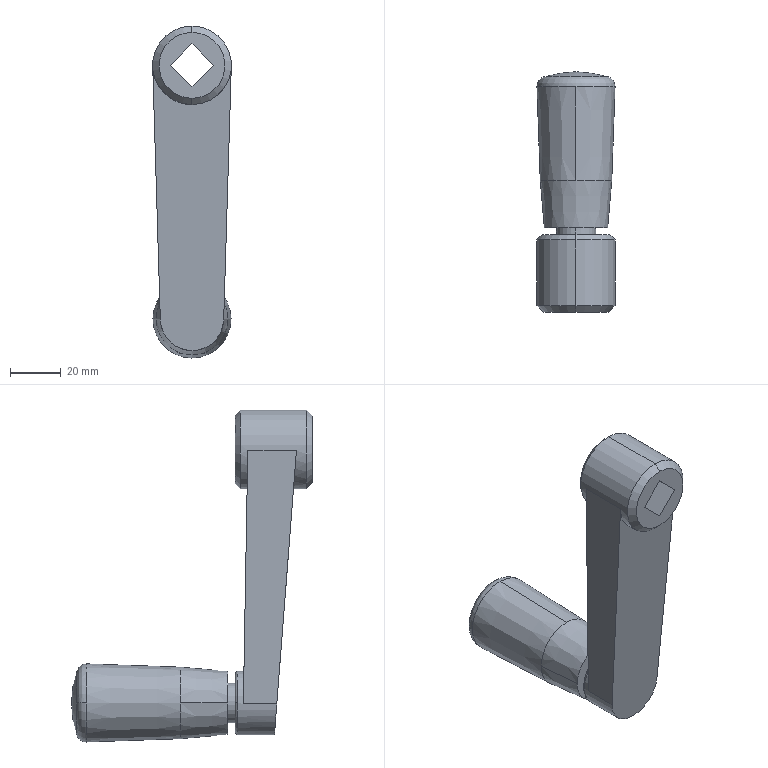Part | SolidWorks | features BaseBody 1 | 1 solid | 34 faces | box 31 x 95 x 130.902 mm | volume 100335 mm3 | plane 13 | cylinder 8 | cone 8 | torus 4 | sphere 1 | commonest cylinder face diameters 15.5 x2 19.799 x2 25 x2 31 x2
STEP:
#1=CARTESIAN_POINT('',(12.494,13.56,-100.375));
#2=VERTEX_POINT('',#1);
#3=CARTESIAN_POINT('',(0.,14.5,-112.5));
#4=VERTEX_POINT('',#3);
#5=CARTESIAN_POINT('',(12.494,13.56,-100.375));
#6=CARTESIAN_POINT('',(12.28,14.114,-107.521));
#7=CARTESIAN_POINT('',(7.149,14.5,-112.5));
#8=CARTESIAN_POINT('',(0.,14.5,-112.5));
#9=(BOUNDED_CURVE()B_SPLINE_CURVE(3,(#5,#6,#7,#8),.UNSPECIFIED.,.F.,.F.)B_SPLINE_CURVE_WITH_KNOTS((4,4),(4.742,6.283),.UNSPECIFIED.)CURVE()GEOMETRIC_REPRESENTATION_ITEM()RATIONAL_B_SPLINE_CURVE((1.,0.8118,0.8118,1.))REPRESENTATION_ITEM(''));
#10=EDGE_CURVE('',#2,#4,#9,.T.);
#11=ORIENTED_EDGE('',*,*,#10,.T.);
#12=CARTESIAN_POINT('',(0.,29.,-112.5));
#13=VERTEX_POINT('',#12);
#14=CARTESIAN_POINT('',(0.,30.,-112.5));
#15=DIRECTION('',(0.,1.,0.));
#16=VECTOR('',#15,1000.);
#17=LINE('',#14,#16);
#18=EDGE_CURVE('',#4,#13,#17,.T.);
#19=ORIENTED_EDGE('',*,*,#18,.T.);
#20=CARTESIAN_POINT('',(12.5,29.,-100.));
#21=VERTEX_POINT('',#20);
#22=CARTESIAN_POINT('',(0.,29.,-100.));
#23=DIRECTION('',(0.,-1.,0.));
#24=DIRECTION('',(0.,0.,1.));
#25=AXIS2_PLACEMENT_3D('',#22,#23,#24);
#26=CIRCLE('',#25,12.5);
#27=EDGE_CURVE('',#13,#21,#26,.T.);
#28=ORIENTED_EDGE('',*,*,#27,.T.);
#29=CARTESIAN_POINT('',(0.,29.,-87.5));
#30=VERTEX_POINT('',#29);
#31=CARTESIAN_POINT('',(0.,29.,-100.));
#32=DIRECTION('',(0.,-1.,0.));
#33=DIRECTION('',(0.,0.,1.));
#34=AXIS2_PLACEMENT_3D('',#31,#32,#33);
#35=CIRCLE('',#34,12.5);
#36=EDGE_CURVE('',#21,#30,#35,.T.);
#37=ORIENTED_EDGE('',*,*,#36,.T.);
#38=CARTESIAN_POINT('',(0.,26.527,-87.5));
#39=VERTEX_POINT('',#38);
#40=CARTESIAN_POINT('',(0.,30.,-87.5));
#41=DIRECTION('',(0.,1.,0.));
#42=VECTOR('',#41,1000.);
#43=LINE('',#40,#42);
#44=EDGE_CURVE('',#39,#30,#43,.T.);
#45=ORIENTED_EDGE('',*,*,#44,.F.);
#46=CARTESIAN_POINT('',(12.494,26.752,-100.375));
#47=VERTEX_POINT('',#46);
#48=CARTESIAN_POINT('',(0.,26.527,-87.5));
#49=CARTESIAN_POINT('',(7.498,26.527,-87.5));
#50=CARTESIAN_POINT('',(12.719,26.621,-92.881));
#51=CARTESIAN_POINT('',(12.494,26.752,-100.375));
#52=(BOUNDED_CURVE()B_SPLINE_CURVE(3,(#48,#49,#50,#51),.UNSPECIFIED.,.F.,.F.)B_SPLINE_CURVE_WITH_KNOTS((4,4),(3.142,4.742),.UNSPECIFIED.)CURVE()GEOMETRIC_REPRESENTATION_ITEM()RATIONAL_B_SPLINE_CURVE((1.,0.7976,0.7976,1.))REPRESENTATION_ITEM(''));
#53=EDGE_CURVE('',#39,#47,#52,.T.);
#54=ORIENTED_EDGE('',*,*,#53,.T.);
#55=CARTESIAN_POINT('',(12.494,30.,-100.375));
#56=DIRECTION('',(0.,-1.,0.));
#57=VECTOR('',#56,1000.);
#58=LINE('',#55,#57);
#59=EDGE_CURVE('',#47,#2,#58,.T.);
#60=ORIENTED_EDGE('',*,*,#59,.T.);
#61=EDGE_LOOP('',(#11,#19,#28,#37,#45,#54,#60));
#62=FACE_OUTER_BOUND('',#61,.T.);
#63=CARTESIAN_POINT('',(0.,30.,-100.));
#64=DIRECTION('',(0.,1.,0.));
#65=DIRECTION('',(0.,0.,1.));
#66=AXIS2_PLACEMENT_3D('',#63,#64,#65);
#67=CYLINDRICAL_SURFACE('',#66,12.5);
#68=ADVANCED_FACE('',(#62),#67,.T.);
#69=CARTESIAN_POINT('',(0.,2.,15.5));
#70=VERTEX_POINT('',#69);
#71=CARTESIAN_POINT('',(0.,2.,-15.5));
#72=VERTEX_POINT('',#71);
#73=CARTESIAN_POINT('',(0.,2.,0.));
#74=DIRECTION('',(0.,1.,0.));
#75=DIRECTION('',(0.,0.,1.));
#76=AXIS2_PLACEMENT_3D('',#73,#74,#75);
#77=CIRCLE('',#76,15.5);
#78=EDGE_CURVE('',#70,#72,#77,.T.);
#79=ORIENTED_EDGE('',*,*,#78,.T.);
#80=CARTESIAN_POINT('',(0.,6.98,-15.5));
#81=VERTEX_POINT('',#80);
#82=CARTESIAN_POINT('',(0.,30.,-15.5));
#83=DIRECTION('',(0.,1.,0.));
#84=VECTOR('',#83,1000.);
#85=LINE('',#82,#84);
#86=EDGE_CURVE('',#72,#81,#85,.T.);
#87=ORIENTED_EDGE('',*,*,#86,.T.);
#88=CARTESIAN_POINT('',(15.493,5.815,-0.465));
#89=VERTEX_POINT('',#88);
#90=CARTESIAN_POINT('',(0.,6.98,-15.5));
#91=CARTESIAN_POINT('',(8.865,6.98,-15.5));
#92=CARTESIAN_POINT('',(15.227,6.502,-9.326));
#93=CARTESIAN_POINT('',(15.493,5.815,-0.465));
#94=(BOUNDED_CURVE()B_SPLINE_CURVE(3,(#90,#91,#92,#93),.UNSPECIFIED.,.F.,.F.)B_SPLINE_CURVE_WITH_KNOTS((4,4),(0.,1.541),.UNSPECIFIED.)CURVE()GEOMETRIC_REPRESENTATION_ITEM()RATIONAL_B_SPLINE_CURVE((1.,0.8118,0.8118,1.))REPRESENTATION_ITEM(''));
#95=EDGE_CURVE('',#81,#89,#94,.T.);
#96=ORIENTED_EDGE('',*,*,#95,.T.);
#97=CARTESIAN_POINT('',(15.493,25.008,-0.465));
#98=VERTEX_POINT('',#97);
#99=CARTESIAN_POINT('',(15.493,30.,-0.465));
#100=DIRECTION('',(0.,1.,0.));
#101=VECTOR('',#100,1000.);
#102=LINE('',#99,#101);
#103=EDGE_CURVE('',#89,#98,#102,.T.);
#104=ORIENTED_EDGE('',*,*,#103,.T.);
#105=CARTESIAN_POINT('',(0.,25.271,-15.5));
#106=VERTEX_POINT('',#105);
#107=CARTESIAN_POINT('',(15.493,25.008,-0.465));
#108=CARTESIAN_POINT('',(15.227,25.163,-9.326));
#109=CARTESIAN_POINT('',(8.865,25.271,-15.5));
#110=CARTESIAN_POINT('',(0.,25.271,-15.5));
#111=(BOUNDED_CURVE()B_SPLINE_CURVE(3,(#107,#108,#109,#110),.UNSPECIFIED.,.F.,.F.)B_SPLINE_CURVE_WITH_KNOTS((4,4),(4.742,6.283),.UNSPECIFIED.)CURVE()GEOMETRIC_REPRESENTATION_ITEM()RATIONAL_B_SPLINE_CURVE((1.,0.8118,0.8118,1.))REPRESENTATION_ITEM(''));
#112=EDGE_CURVE('',#98,#106,#111,.T.);
#113=ORIENTED_EDGE('',*,*,#112,.T.);
#114=CARTESIAN_POINT('',(0.,28.,-15.5));
#115=VERTEX_POINT('',#114);
#116=CARTESIAN_POINT('',(0.,30.,-15.5));
#117=DIRECTION('',(0.,1.,0.));
#118=VECTOR('',#117,1000.);
#119=LINE('',#116,#118);
#120=EDGE_CURVE('',#106,#115,#119,.T.);
#121=ORIENTED_EDGE('',*,*,#120,.T.);
#122=CARTESIAN_POINT('',(0.,28.,15.5));
#123=VERTEX_POINT('',#122);
#124=CARTESIAN_POINT('',(0.,28.,0.));
#125=DIRECTION('',(0.,-1.,0.));
#126=DIRECTION('',(0.,0.,1.));
#127=AXIS2_PLACEMENT_3D('',#124,#125,#126);
#128=CIRCLE('',#127,15.5);
#129=EDGE_CURVE('',#115,#123,#128,.T.);
#130=ORIENTED_EDGE('',*,*,#129,.T.);
#131=CARTESIAN_POINT('',(0.,30.,15.5));
#132=DIRECTION('',(0.,1.,0.));
#133=VECTOR('',#132,1000.);
#134=LINE('',#131,#133);
#135=EDGE_CURVE('',#70,#123,#134,.T.);
#136=ORIENTED_EDGE('',*,*,#135,.F.);
#137=EDGE_LOOP('',(#79,#87,#96,#104,#113,#121,#130,#136));
#138=FACE_OUTER_BOUND('',#137,.T.);
#139=CARTESIAN_POINT('',(0.,30.,0.));
#140=DIRECTION('',(0.,1.,0.));
#141=DIRECTION('',(0.,0.,1.));
#142=AXIS2_PLACEMENT_3D('',#139,#140,#141);
#143=CYLINDRICAL_SURFACE('',#142,15.5);
#144=ADVANCED_FACE('',(#138),#143,.T.);
#145=CARTESIAN_POINT('',(0.,30.,-88.5));
#146=VERTEX_POINT('',#145);
#147=CARTESIAN_POINT('',(-11.5,30.,-100.));
#148=VERTEX_POINT('',#147);
#149=CARTESIAN_POINT('',(0.,30.,-100.));
#150=DIRECTION('',(0.,-1.,0.));
#151=DIRECTION('',(1.,0.,0.));
#152=AXIS2_PLACEMENT_3D('',#149,#150,#151);
#153=CIRCLE('',#152,11.5);
#154=EDGE_CURVE('',#146,#148,#153,.T.);
#155=ORIENTED_EDGE('',*,*,#154,.T.);
#156=CARTESIAN_POINT('',(-12.5,29.,-100.));
#157=VERTEX_POINT('',#156);
#158=CARTESIAN_POINT('',(-11.5,29.,-100.));
#159=DIRECTION('',(0.,0.,1.));
#160=DIRECTION('',(1.,0.,0.));
#161=AXIS2_PLACEMENT_3D('',#158,#159,#160);
#162=CIRCLE('',#161,1.);
#163=EDGE_CURVE('',#148,#157,#162,.T.);
#164=ORIENTED_EDGE('',*,*,#163,.T.);
#165=CARTESIAN_POINT('',(0.,29.,-100.));
#166=DIRECTION('',(0.,-1.,0.));
#167=DIRECTION('',(0.,0.,1.));
#168=AXIS2_PLACEMENT_3D('',#165,#166,#167);
#169=CIRCLE('',#168,12.5);
#170=EDGE_CURVE('',#30,#157,#169,.T.);
#171=ORIENTED_EDGE('',*,*,#170,.F.);
#172=ORIENTED_EDGE('',*,*,#36,.F.);
#173=CARTESIAN_POINT('',(11.5,30.,-100.));
#174=VERTEX_POINT('',#173);
#175=CARTESIAN_POINT('',(11.5,29.,-100.));
#176=DIRECTION('',(0.,0.,-1.));
#177=DIRECTION('',(0.,1.,0.));
#178=AXIS2_PLACEMENT_3D('',#175,#176,#177);
#179=CIRCLE('',#178,1.);
#180=EDGE_CURVE('',#174,#21,#179,.T.);
#181=ORIENTED_EDGE('',*,*,#180,.F.);
#182=CARTESIAN_POINT('',(11.5,30.,-100.));
#183=CARTESIAN_POINT('',(11.5,30.,-98.495));
#184=CARTESIAN_POINT('',(11.201,30.,-96.99));
#185=CARTESIAN_POINT('',(10.049,30.,-94.208));
#186=CARTESIAN_POINT('',(9.196,30.,-92.933));
#187=CARTESIAN_POINT('',(7.067,30.,-90.804));
#188=CARTESIAN_POINT('',(5.792,30.,-89.951));
#189=CARTESIAN_POINT('',(3.01,30.,-88.799));
#190=CARTESIAN_POINT('',(1.505,30.,-88.5));
#191=CARTESIAN_POINT('',(0.,30.,-88.5));
#192=B_SPLINE_CURVE_WITH_KNOTS('',3,(#182,#183,#184,#185,#186,#187,#188,#189,#190,#191),.UNSPECIFIED.,.F.,.F.,(4,2,2,2,4),(0.5,0.625,0.75,0.875,1.),.UNSPECIFIED.);
#193=EDGE_CURVE('',#174,#146,#192,.T.);
#194=ORIENTED_EDGE('',*,*,#193,.T.);
#195=EDGE_LOOP('',(#155,#164,#171,#172,#181,#194));
#196=FACE_OUTER_BOUND('',#195,.T.);
#197=CARTESIAN_POINT('',(0.,29.,-100.));
#198=DIRECTION('',(0.,-1.,0.));
#199=DIRECTION('',(1.,0.,0.));
#200=AXIS2_PLACEMENT_3D('',#197,#198,#199);
#201=TOROIDAL_SURFACE('',#200,11.5,1.);
#202=ADVANCED_FACE('',(#196),#201,.T.);
#203=CARTESIAN_POINT('',(0.,30.,-13.5));
#204=VERTEX_POINT('',#203);
#205=CARTESIAN_POINT('',(0.,30.,13.5));
#206=VERTEX_POINT('',#205);
#207=CARTESIAN_POINT('',(0.,30.,0.));
#208=DIRECTION('',(0.,-1.,0.));
#209=DIRECTION('',(0.,0.,-1.));
#210=AXIS2_PLACEMENT_3D('',#207,#208,#209);
#211=CIRCLE('',#210,13.5);
#212=EDGE_CURVE('',#204,#206,#211,.T.);
#213=ORIENTED_EDGE('',*,*,#212,.T.);
#214=CARTESIAN_POINT('',(0.,28.,15.5));
#215=DIRECTION('',(0.,-0.7071,0.7071));
#216=VECTOR('',#215,1000.);
#217=LINE('',#214,#216);
#218=EDGE_CURVE('',#206,#123,#217,.T.);
#219=ORIENTED_EDGE('',*,*,#218,.T.);
#220=ORIENTED_EDGE('',*,*,#129,.F.);
#221=CARTESIAN_POINT('',(0.,28.,-15.5));
#222=DIRECTION('',(0.,-0.7071,-0.7071));
#223=VECTOR('',#222,1000.);
#224=LINE('',#221,#223);
#225=EDGE_CURVE('',#204,#115,#224,.T.);
#226=ORIENTED_EDGE('',*,*,#225,.F.);
#227=EDGE_LOOP('',(#213,#219,#220,#226));
#228=FACE_OUTER_BOUND('',#227,.T.);
#229=CARTESIAN_POINT('',(0.,28.,0.));
#230=DIRECTION('',(0.,-1.,0.));
#231=DIRECTION('',(0.,0.,-1.));
#232=AXIS2_PLACEMENT_3D('',#229,#230,#231);
#233=CONICAL_SURFACE('',#232,15.5,0.7854);
#234=ADVANCED_FACE('',(#228),#233,.T.);
#235=CARTESIAN_POINT('',(0.,-0.5,13.));
#236=VERTEX_POINT('',#235);
#237=CARTESIAN_POINT('',(0.,-0.5,-13.));
#238=VERTEX_POINT('',#237);
#239=CARTESIAN_POINT('',(0.,-0.5,0.));
#240=DIRECTION('',(0.,1.,0.));
#241=DIRECTION('',(0.,0.,1.));
#242=AXIS2_PLACEMENT_3D('',#239,#240,#241);
#243=CIRCLE('',#242,13.);
#244=EDGE_CURVE('',#236,#238,#243,.T.);
#245=ORIENTED_EDGE('',*,*,#244,.T.);
#246=CARTESIAN_POINT('',(0.,2.,-15.5));
#247=DIRECTION('',(0.,0.7071,-0.7071));
#248=VECTOR('',#247,1000.);
#249=LINE('',#246,#248);
#250=EDGE_CURVE('',#238,#72,#249,.T.);
#251=ORIENTED_EDGE('',*,*,#250,.T.);
#252=ORIENTED_EDGE('',*,*,#78,.F.);
#253=CARTESIAN_POINT('',(0.,2.,15.5));
#254=DIRECTION('',(0.,0.7071,0.7071));
#255=VECTOR('',#254,1000.);
#256=LINE('',#253,#255);
#257=EDGE_CURVE('',#236,#70,#256,.T.);
#258=ORIENTED_EDGE('',*,*,#257,.F.);
#259=EDGE_LOOP('',(#245,#251,#252,#258));
#260=FACE_OUTER_BOUND('',#259,.T.);
#261=CARTESIAN_POINT('',(0.,2.,0.));
#262=DIRECTION('',(0.,1.,0.));
#263=DIRECTION('',(0.,0.,1.));
#264=AXIS2_PLACEMENT_3D('',#261,#262,#263);
#265=CONICAL_SURFACE('',#264,15.5,0.7854);
#266=ADVANCED_FACE('',(#260),#265,.T.);
#267=CARTESIAN_POINT('',(0.,30.,-92.25));
#268=VERTEX_POINT('',#267);
#269=CARTESIAN_POINT('',(0.,30.,-107.75));
#270=VERTEX_POINT('',#269);
#271=CARTESIAN_POINT('',(0.,30.,-100.));
#272=DIRECTION('',(0.,1.,0.));
#273=DIRECTION('',(0.,0.,1.));
#274=AXIS2_PLACEMENT_3D('',#271,#272,#273);
#275=CIRCLE('',#274,7.75);
#276=EDGE_CURVE('',#268,#270,#275,.T.);
#277=ORIENTED_EDGE('',*,*,#276,.T.);
#278=CARTESIAN_POINT('',(0.,33.,-107.75));
#279=VERTEX_POINT('',#278);
#280=CARTESIAN_POINT('',(0.,30.,-107.75));
#281=DIRECTION('',(0.,1.,0.));
#282=VECTOR('',#281,1000.);
#283=LINE('',#280,#282);
#284=EDGE_CURVE('',#270,#279,#283,.T.);
#285=ORIENTED_EDGE('',*,*,#284,.T.);
#286=CARTESIAN_POINT('',(0.,33.,-92.25));
#287=VERTEX_POINT('',#286);
#288=CARTESIAN_POINT('',(0.,33.,-100.));
#289=DIRECTION('',(0.,-1.,0.));
#290=DIRECTION('',(0.,0.,1.));
#291=AXIS2_PLACEMENT_3D('',#288,#289,#290);
#292=CIRCLE('',#291,7.75);
#293=EDGE_CURVE('',#279,#287,#292,.T.);
#294=ORIENTED_EDGE('',*,*,#293,.T.);
#295=CARTESIAN_POINT('',(0.,30.,-92.25));
#296=DIRECTION('',(0.,1.,0.));
#297=VECTOR('',#296,1000.);
#298=LINE('',#295,#297);
#299=EDGE_CURVE('',#268,#287,#298,.T.);
#300=ORIENTED_EDGE('',*,*,#299,.F.);
#301=EDGE_LOOP('',(#277,#285,#294,#300));
#302=FACE_OUTER_BOUND('',#301,.T.);
#303=CARTESIAN_POINT('',(0.,30.,-100.));
#304=DIRECTION('',(0.,1.,0.));
#305=DIRECTION('',(0.,0.,1.));
#306=AXIS2_PLACEMENT_3D('',#303,#304,#305);
#307=CYLINDRICAL_SURFACE('',#306,7.75);
#308=ADVANCED_FACE('',(#302),#307,.T.);
#309=CARTESIAN_POINT('',(0.,26.5,-9.899));
#310=VERTEX_POINT('',#309);
#311=CARTESIAN_POINT('',(0.,26.5,9.899));
#312=VERTEX_POINT('',#311);
#313=CARTESIAN_POINT('',(0.,26.5,0.));
#314=DIRECTION('',(0.,1.,0.));
#315=DIRECTION('',(0.,0.,1.));
#316=AXIS2_PLACEMENT_3D('',#313,#314,#315);
#317=CIRCLE('',#316,9.899);
#318=EDGE_CURVE('',#310,#312,#317,.T.);
#319=ORIENTED_EDGE('',*,*,#318,.F.);
#320=CARTESIAN_POINT('',(0.,30.,-9.899));
#321=VERTEX_POINT('',#320);
#322=CARTESIAN_POINT('',(0.,33.5,-9.899));
#323=DIRECTION('',(0.,1.,0.));
#324=VECTOR('',#323,1000.);
#325=LINE('',#322,#324);
#326=EDGE_CURVE('',#310,#321,#325,.T.);
#327=ORIENTED_EDGE('',*,*,#326,.T.);
#328=CARTESIAN_POINT('',(0.,30.,9.899));
#329=VERTEX_POINT('',#328);
#330=CARTESIAN_POINT('',(0.,30.,0.));
#331=DIRECTION('',(0.,1.,0.));
#332=DIRECTION('',(0.,0.,1.));
#333=AXIS2_PLACEMENT_3D('',#330,#331,#332);
#334=CIRCLE('',#333,9.899);
#335=EDGE_CURVE('',#321,#329,#334,.T.);
#336=ORIENTED_EDGE('',*,*,#335,.T.);
#337=CARTESIAN_POINT('',(0.,33.5,9.899));
#338=DIRECTION('',(0.,1.,0.));
#339=VECTOR('',#338,1000.);
#340=LINE('',#337,#339);
#341=EDGE_CURVE('',#312,#329,#340,.T.);
#342=ORIENTED_EDGE('',*,*,#341,.F.);
#343=EDGE_LOOP('',(#319,#327,#336,#342));
#344=FACE_OUTER_BOUND('',#343,.T.);
#345=CARTESIAN_POINT('',(0.,33.5,0.));
#346=DIRECTION('',(0.,1.,0.));
#347=DIRECTION('',(0.,0.,1.));
#348=AXIS2_PLACEMENT_3D('',#345,#346,#347);
#349=CYLINDRICAL_SURFACE('',#348,9.899);
#350=ADVANCED_FACE('',(#344),#349,.F.);
#351=CARTESIAN_POINT('',(-12.488,33.,-100.));
#352=VERTEX_POINT('',#351);
#353=CARTESIAN_POINT('',(12.488,33.,-100.));
#354=VERTEX_POINT('',#353);
#355=CARTESIAN_POINT('',(0.,33.,-100.));
#356=DIRECTION('',(0.,1.,0.));
#357=DIRECTION('',(-1.,0.,0.));
#358=AXIS2_PLACEMENT_3D('',#355,#356,#357);
#359=CIRCLE('',#358,12.488);
#360=EDGE_CURVE('',#352,#354,#359,.T.);
#361=ORIENTED_EDGE('',*,*,#360,.T.);
#362=CARTESIAN_POINT('',(14.107,51.5,-100.));
#363=VERTEX_POINT('',#362);
#364=CARTESIAN_POINT('',(14.107,51.5,-100.));
#365=DIRECTION('',(0.08716,0.9962,0.));
#366=VECTOR('',#365,1000.);
#367=LINE('',#364,#366);
#368=EDGE_CURVE('',#354,#363,#367,.T.);
#369=ORIENTED_EDGE('',*,*,#368,.T.);
#370=CARTESIAN_POINT('',(0.,51.5,-85.893));
#371=VERTEX_POINT('',#370);
#372=CARTESIAN_POINT('',(0.,51.5,-100.));
#373=DIRECTION('',(0.,-1.,0.));
#374=DIRECTION('',(0.,0.,1.));
#375=AXIS2_PLACEMENT_3D('',#372,#373,#374);
#376=CIRCLE('',#375,14.107);
#377=EDGE_CURVE('',#363,#371,#376,.T.);
#378=ORIENTED_EDGE('',*,*,#377,.T.);
#379=CARTESIAN_POINT('',(-14.107,51.5,-100.));
#380=VERTEX_POINT('',#379);
#381=CARTESIAN_POINT('',(0.,51.5,-100.));
#382=DIRECTION('',(0.,-1.,0.));
#383=DIRECTION('',(0.,0.,1.));
#384=AXIS2_PLACEMENT_3D('',#381,#382,#383);
#385=CIRCLE('',#384,14.107);
#386=EDGE_CURVE('',#371,#380,#385,.T.);
#387=ORIENTED_EDGE('',*,*,#386,.T.);
#388=CARTESIAN_POINT('',(-14.107,51.5,-100.));
#389=DIRECTION('',(-0.08716,0.9962,0.));
#390=VECTOR('',#389,1000.);
#391=LINE('',#388,#390);
#392=EDGE_CURVE('',#352,#380,#391,.T.);
#393=ORIENTED_EDGE('',*,*,#392,.F.);
#394=EDGE_LOOP('',(#361,#369,#378,#387,#393));
#395=FACE_OUTER_BOUND('',#394,.T.);
#396=CARTESIAN_POINT('',(0.,51.5,-100.));
#397=DIRECTION('',(0.,1.,0.));
#398=DIRECTION('',(-1.,0.,0.));
#399=AXIS2_PLACEMENT_3D('',#396,#397,#398);
#400=CONICAL_SURFACE('',#399,14.107,0.08727);
#401=ADVANCED_FACE('',(#395),#400,.T.);
#402=CARTESIAN_POINT('',(0.,51.5,-114.107));
#403=VERTEX_POINT('',#402);
#404=CARTESIAN_POINT('',(0.,51.5,-100.));
#405=DIRECTION('',(0.,-1.,0.));
#406=DIRECTION('',(0.,0.,1.));
#407=AXIS2_PLACEMENT_3D('',#404,#405,#406);
#408=CIRCLE('',#407,14.107);
#409=EDGE_CURVE('',#403,#363,#408,.T.);
#410=ORIENTED_EDGE('',*,*,#409,.F.);
#411=CARTESIAN_POINT('',(0.,88.523,-115.4));
#412=VERTEX_POINT('',#411);
#413=CARTESIAN_POINT('',(0.,88.523,-115.4));
#414=DIRECTION('',(0.,0.9994,-0.0349));
#415=VECTOR('',#414,1000.);
#416=LINE('',#413,#415);
#417=EDGE_CURVE('',#403,#412,#416,.T.);
#418=ORIENTED_EDGE('',*,*,#417,.T.);
#419=CARTESIAN_POINT('',(15.4,88.523,-100.));
#420=VERTEX_POINT('',#419);
#421=CARTESIAN_POINT('',(0.,88.523,-100.));
#422=DIRECTION('',(0.,-1.,0.));
#423=DIRECTION('',(0.,0.,1.));
#424=AXIS2_PLACEMENT_3D('',#421,#422,#423);
#425=CIRCLE('',#424,15.4);
#426=EDGE_CURVE('',#412,#420,#425,.T.);
#427=ORIENTED_EDGE('',*,*,#426,.T.);
#428=CARTESIAN_POINT('',(0.,88.523,-84.6));
#429=VERTEX_POINT('',#428);
#430=CARTESIAN_POINT('',(0.,88.523,-100.));
#431=DIRECTION('',(0.,-1.,0.));
#432=DIRECTION('',(0.,0.,1.));
#433=AXIS2_PLACEMENT_3D('',#430,#431,#432);
#434=CIRCLE('',#433,15.4);
#435=EDGE_CURVE('',#420,#429,#434,.T.);
#436=ORIENTED_EDGE('',*,*,#435,.T.);
#437=CARTESIAN_POINT('',(0.,88.523,-84.6));
#438=DIRECTION('',(0.,0.9994,0.0349));
#439=VECTOR('',#438,1000.);
#440=LINE('',#437,#439);
#441=EDGE_CURVE('',#371,#429,#440,.T.);
#442=ORIENTED_EDGE('',*,*,#441,.F.);
#443=ORIENTED_EDGE('',*,*,#377,.F.);
#444=EDGE_LOOP('',(#410,#418,#427,#436,#442,#443));
#445=FACE_OUTER_BOUND('',#444,.T.);
#446=CARTESIAN_POINT('',(0.,88.523,-100.));
#447=DIRECTION('',(0.,1.,0.));
#448=DIRECTION('',(0.,0.,1.));
#449=AXIS2_PLACEMENT_3D('',#446,#447,#448);
#450=CONICAL_SURFACE('',#449,15.4,0.03491);
#451=ADVANCED_FACE('',(#445),#450,.T.);
#452=CARTESIAN_POINT('',(12.658,92.46,-100.));
#453=VERTEX_POINT('',#452);
#454=CARTESIAN_POINT('',(-12.658,92.46,-100.));
#455=VERTEX_POINT('',#454);
#456=CARTESIAN_POINT('',(0.,92.46,-100.));
#457=DIRECTION('',(0.,-1.,0.));
#458=DIRECTION('',(0.,0.,-1.));
#459=AXIS2_PLACEMENT_3D('',#456,#457,#458);
#460=CIRCLE('',#459,12.658);
#461=EDGE_CURVE('',#453,#455,#460,.T.);
#462=ORIENTED_EDGE('',*,*,#461,.T.);
#463=CARTESIAN_POINT('',(-15.4,88.523,-100.));
#464=VERTEX_POINT('',#463);
#465=CARTESIAN_POINT('',(-11.402,88.663,-100.));
#466=DIRECTION('',(0.,0.,1.));
#467=DIRECTION('',(1.,0.,0.));
#468=AXIS2_PLACEMENT_3D('',#465,#466,#467);
#469=CIRCLE('',#468,4.);
#470=EDGE_CURVE('',#455,#464,#469,.T.);
#471=ORIENTED_EDGE('',*,*,#470,.T.);
#472=CARTESIAN_POINT('',(0.,88.523,-100.));
#473=DIRECTION('',(0.,-1.,0.));
#474=DIRECTION('',(0.,0.,1.));
#475=AXIS2_PLACEMENT_3D('',#472,#473,#474);
#476=CIRCLE('',#475,15.4);
#477=EDGE_CURVE('',#429,#464,#476,.T.);
#478=ORIENTED_EDGE('',*,*,#477,.F.);
#479=ORIENTED_EDGE('',*,*,#435,.F.);
#480=CARTESIAN_POINT('',(11.402,88.663,-100.));
#481=DIRECTION('',(0.,0.,-1.));
#482=DIRECTION('',(-1.,0.,0.));
#483=AXIS2_PLACEMENT_3D('',#480,#481,#482);
#484=CIRCLE('',#483,4.);
#485=EDGE_CURVE('',#453,#420,#484,.T.);
#486=ORIENTED_EDGE('',*,*,#485,.F.);
#487=EDGE_LOOP('',(#462,#471,#478,#479,#486));
#488=FACE_OUTER_BOUND('',#487,.T.);
#489=CARTESIAN_POINT('',(0.,88.663,-100.));
#490=DIRECTION('',(0.,-1.,0.));
#491=DIRECTION('',(1.,0.,0.));
#492=AXIS2_PLACEMENT_3D('',#489,#490,#491);
#493=TOROIDAL_SURFACE('',#492,11.402,4.);
#494=ADVANCED_FACE('',(#488),#493,.T.);
#495=CARTESIAN_POINT('',(-12.494,13.56,-100.375));
#496=VERTEX_POINT('',#495);
#497=CARTESIAN_POINT('',(-15.493,5.815,-0.465));
#498=VERTEX_POINT('',#497);
#499=CARTESIAN_POINT('',(-12.494,13.56,-100.375));
#500=DIRECTION('',(-0.02991,-0.07726,0.9966));
#501=VECTOR('',#500,1000.);
#502=LINE('',#499,#501);
#503=EDGE_CURVE('',#496,#498,#502,.T.);
#504=ORIENTED_EDGE('',*,*,#503,.F.);
#505=CARTESIAN_POINT('',(0.,14.5,-112.5));
#506=CARTESIAN_POINT('',(-7.149,14.5,-112.5));
#507=CARTESIAN_POINT('',(-12.28,14.114,-107.521));
#508=CARTESIAN_POINT('',(-12.494,13.56,-100.375));
#509=(BOUNDED_CURVE()B_SPLINE_CURVE(3,(#505,#506,#507,#508),.UNSPECIFIED.,.F.,.F.)B_SPLINE_CURVE_WITH_KNOTS((4,4),(0.,1.541),.UNSPECIFIED.)CURVE()GEOMETRIC_REPRESENTATION_ITEM()RATIONAL_B_SPLINE_CURVE((1.,0.8118,0.8118,1.))REPRESENTATION_ITEM(''));
#510=EDGE_CURVE('',#4,#496,#509,.T.);
#511=ORIENTED_EDGE('',*,*,#510,.F.);
#512=ORIENTED_EDGE('',*,*,#10,.F.);
#513=CARTESIAN_POINT('',(15.493,5.815,-0.465));
#514=DIRECTION('',(-0.02991,0.07726,-0.9966));
#515=VECTOR('',#514,1000.);
#516=LINE('',#513,#515);
#517=EDGE_CURVE('',#89,#2,#516,.T.);
#518=ORIENTED_EDGE('',*,*,#517,.F.);
#519=ORIENTED_EDGE('',*,*,#95,.F.);
#520=CARTESIAN_POINT('',(-15.493,5.815,-0.465));
#521=CARTESIAN_POINT('',(-15.227,6.502,-9.326));
#522=CARTESIAN_POINT('',(-8.865,6.98,-15.5));
#523=CARTESIAN_POINT('',(0.,6.98,-15.5));
#524=(BOUNDED_CURVE()B_SPLINE_CURVE(3,(#520,#521,#522,#523),.UNSPECIFIED.,.F.,.F.)B_SPLINE_CURVE_WITH_KNOTS((4,4),(4.742,6.283),.UNSPECIFIED.)CURVE()GEOMETRIC_REPRESENTATION_ITEM()RATIONAL_B_SPLINE_CURVE((1.,0.8118,0.8118,1.))REPRESENTATION_ITEM(''));
#525=EDGE_CURVE('',#498,#81,#524,.T.);
#526=ORIENTED_EDGE('',*,*,#525,.F.);
#527=EDGE_LOOP('',(#504,#511,#512,#518,#519,#526));
#528=FACE_OUTER_BOUND('',#527,.T.);
#529=CARTESIAN_POINT('',(100.,3.375,31.));
#530=DIRECTION('',(0.,0.997,0.07729));
#531=DIRECTION('',(0.,-0.07729,0.997));
#532=AXIS2_PLACEMENT_3D('',#529,#530,#531);
#533=PLANE('',#532);
#534=ADVANCED_FACE('',(#528),#533,.F.);
#535=CARTESIAN_POINT('',(-12.494,26.752,-100.375));
#536=VERTEX_POINT('',#535);
#537=CARTESIAN_POINT('',(-12.494,30.,-100.375));
#538=DIRECTION('',(0.,1.,0.));
#539=VECTOR('',#538,1000.);
#540=LINE('',#537,#539);
#541=EDGE_CURVE('',#496,#536,#540,.T.);
#542=ORIENTED_EDGE('',*,*,#541,.F.);
#543=ORIENTED_EDGE('',*,*,#503,.T.);
#544=CARTESIAN_POINT('',(-15.493,25.008,-0.465));
#545=VERTEX_POINT('',#544);
#546=CARTESIAN_POINT('',(-15.493,30.,-0.465));
#547=DIRECTION('',(0.,-1.,0.));
#548=VECTOR('',#547,1000.);
#549=LINE('',#546,#548);
#550=EDGE_CURVE('',#545,#498,#549,.T.);
#551=ORIENTED_EDGE('',*,*,#550,.F.);
#552=CARTESIAN_POINT('',(-12.494,26.752,-100.375));
#553=DIRECTION('',(-0.03,-0.01744,0.9994));
#554=VECTOR('',#553,1000.);
#555=LINE('',#552,#554);
#556=EDGE_CURVE('',#536,#545,#555,.T.);
#557=ORIENTED_EDGE('',*,*,#556,.F.);
#558=EDGE_LOOP('',(#542,#543,#551,#557));
#559=FACE_OUTER_BOUND('',#558,.T.);
#560=CARTESIAN_POINT('',(-12.494,30.,-100.375));
#561=DIRECTION('',(0.9995,0.,0.03));
#562=DIRECTION('',(0.03,0.,-0.9995));
#563=AXIS2_PLACEMENT_3D('',#560,#561,#562);
#564=PLANE('',#563);
#565=ADVANCED_FACE('',(#559),#564,.F.);
#566=ORIENTED_EDGE('',*,*,#18,.F.);
#567=ORIENTED_EDGE('',*,*,#510,.T.);
#568=ORIENTED_EDGE('',*,*,#541,.T.);
#569=CARTESIAN_POINT('',(-12.494,26.752,-100.375));
#570=CARTESIAN_POINT('',(-12.719,26.621,-92.881));
#571=CARTESIAN_POINT('',(-7.498,26.527,-87.5));
#572=CARTESIAN_POINT('',(0.,26.527,-87.5));
#573=(BOUNDED_CURVE()B_SPLINE_CURVE(3,(#569,#570,#571,#572),.UNSPECIFIED.,.F.,.F.)B_SPLINE_CURVE_WITH_KNOTS((4,4),(1.541,3.142),.UNSPECIFIED.)CURVE()GEOMETRIC_REPRESENTATION_ITEM()RATIONAL_B_SPLINE_CURVE((1.,0.7976,0.7976,1.))REPRESENTATION_ITEM(''));
#574=EDGE_CURVE('',#536,#39,#573,.T.);
#575=ORIENTED_EDGE('',*,*,#574,.T.);
#576=ORIENTED_EDGE('',*,*,#44,.T.);
#577=ORIENTED_EDGE('',*,*,#170,.T.);
#578=CARTESIAN_POINT('',(0.,29.,-100.));
#579=DIRECTION('',(0.,-1.,0.));
#580=DIRECTION('',(0.,0.,1.));
#581=AXIS2_PLACEMENT_3D('',#578,#579,#580);
#582=CIRCLE('',#581,12.5);
#583=EDGE_CURVE('',#157,#13,#582,.T.);
#584=ORIENTED_EDGE('',*,*,#583,.T.);
#585=EDGE_LOOP('',(#566,#567,#568,#575,#576,#577,#584));
#586=FACE_OUTER_BOUND('',#585,.T.);
#587=CARTESIAN_POINT('',(0.,30.,-100.));
#588=DIRECTION('',(0.,1.,0.));
#589=DIRECTION('',(0.,0.,1.));
#590=AXIS2_PLACEMENT_3D('',#587,#588,#589);
#591=CYLINDRICAL_SURFACE('',#590,12.5);
#592=ADVANCED_FACE('',(#586),#591,.T.);
#593=ORIENTED_EDGE('',*,*,#103,.F.);
#594=ORIENTED_EDGE('',*,*,#517,.T.);
#595=ORIENTED_EDGE('',*,*,#59,.F.);
#596=CARTESIAN_POINT('',(15.493,25.008,-0.465));
#597=DIRECTION('',(-0.03,0.01744,-0.9994));
#598=VECTOR('',#597,1000.);
#599=LINE('',#596,#598);
#600=EDGE_CURVE('',#98,#47,#599,.T.);
#601=ORIENTED_EDGE('',*,*,#600,.F.);
#602=EDGE_LOOP('',(#593,#594,#595,#601));
#603=FACE_OUTER_BOUND('',#602,.T.);
#604=CARTESIAN_POINT('',(15.493,30.,-0.465));
#605=DIRECTION('',(-0.9995,0.,0.03));
#606=DIRECTION('',(0.03,0.,0.9995));
#607=AXIS2_PLACEMENT_3D('',#604,#605,#606);
#608=PLANE('',#607);
#609=ADVANCED_FACE('',(#603),#608,.F.);
#610=ORIENTED_EDGE('',*,*,#86,.F.);
#611=CARTESIAN_POINT('',(0.,2.,0.));
#612=DIRECTION('',(0.,1.,0.));
#613=DIRECTION('',(0.,0.,1.));
#614=AXIS2_PLACEMENT_3D('',#611,#612,#613);
#615=CIRCLE('',#614,15.5);
#616=EDGE_CURVE('',#72,#70,#615,.T.);
#617=ORIENTED_EDGE('',*,*,#616,.T.);
#618=ORIENTED_EDGE('',*,*,#135,.T.);
#619=CARTESIAN_POINT('',(0.,28.,0.));
#620=DIRECTION('',(0.,-1.,0.));
#621=DIRECTION('',(0.,0.,1.));
#622=AXIS2_PLACEMENT_3D('',#619,#620,#621);
#623=CIRCLE('',#622,15.5);
#624=EDGE_CURVE('',#123,#115,#623,.T.);
#625=ORIENTED_EDGE('',*,*,#624,.T.);
#626=ORIENTED_EDGE('',*,*,#120,.F.);
#627=CARTESIAN_POINT('',(0.,25.271,-15.5));
#628=CARTESIAN_POINT('',(-8.865,25.271,-15.5));
#629=CARTESIAN_POINT('',(-15.227,25.163,-9.326));
#630=CARTESIAN_POINT('',(-15.493,25.008,-0.465));
#631=(BOUNDED_CURVE()B_SPLINE_CURVE(3,(#627,#628,#629,#630),.UNSPECIFIED.,.F.,.F.)B_SPLINE_CURVE_WITH_KNOTS((4,4),(0.,1.541),.UNSPECIFIED.)CURVE()GEOMETRIC_REPRESENTATION_ITEM()RATIONAL_B_SPLINE_CURVE((1.,0.8118,0.8118,1.))REPRESENTATION_ITEM(''));
#632=EDGE_CURVE('',#106,#545,#631,.T.);
#633=ORIENTED_EDGE('',*,*,#632,.T.);
#634=ORIENTED_EDGE('',*,*,#550,.T.);
#635=ORIENTED_EDGE('',*,*,#525,.T.);
#636=EDGE_LOOP('',(#610,#617,#618,#625,#626,#633,#634,#635));
#637=FACE_OUTER_BOUND('',#636,.T.);
#638=CARTESIAN_POINT('',(0.,30.,0.));
#639=DIRECTION('',(0.,1.,0.));
#640=DIRECTION('',(0.,0.,1.));
#641=AXIS2_PLACEMENT_3D('',#638,#639,#640);
#642=CYLINDRICAL_SURFACE('',#641,15.5);
#643=ADVANCED_FACE('',(#637),#642,.T.);
#644=ORIENTED_EDGE('',*,*,#556,.T.);
#645=ORIENTED_EDGE('',*,*,#632,.F.);
#646=ORIENTED_EDGE('',*,*,#112,.F.);
#647=ORIENTED_EDGE('',*,*,#600,.T.);
#648=ORIENTED_EDGE('',*,*,#53,.F.);
#649=ORIENTED_EDGE('',*,*,#574,.F.);
#650=EDGE_LOOP('',(#644,#645,#646,#647,#648,#649));
#651=FACE_OUTER_BOUND('',#650,.T.);
#652=CARTESIAN_POINT('',(100.,26.964,-112.5));
#653=DIRECTION('',(0.,-0.9998,-0.01745));
#654=DIRECTION('',(0.,0.01745,-0.9998));
#655=AXIS2_PLACEMENT_3D('',#652,#653,#654);
#656=PLANE('',#655);
#657=ADVANCED_FACE('',(#651),#656,.F.);
#658=ORIENTED_EDGE('',*,*,#163,.F.);
#659=CARTESIAN_POINT('',(0.,30.,-111.5));
#660=VERTEX_POINT('',#659);
#661=CARTESIAN_POINT('',(0.,30.,-100.));
#662=DIRECTION('',(0.,-1.,0.));
#663=DIRECTION('',(1.,0.,0.));
#664=AXIS2_PLACEMENT_3D('',#661,#662,#663);
#665=CIRCLE('',#664,11.5);
#666=EDGE_CURVE('',#148,#660,#665,.T.);
#667=ORIENTED_EDGE('',*,*,#666,.T.);
#668=CARTESIAN_POINT('',(0.,30.,-111.5));
#669=CARTESIAN_POINT('',(0.2719,30.,-111.5));
#670=CARTESIAN_POINT('',(0.5439,30.,-111.49));
#671=CARTESIAN_POINT('',(0.9508,30.,-111.462));
#672=CARTESIAN_POINT('',(1.154,30.,-111.444));
#673=CARTESIAN_POINT('',(1.39,30.,-111.416));
#674=CARTESIAN_POINT('',(1.508,30.,-111.401));
#675=CARTESIAN_POINT('',(1.567,30.,-111.393));
#676=CARTESIAN_POINT('',(1.597,30.,-111.389));
#677=CARTESIAN_POINT('',(1.612,30.,-111.387));
#678=CARTESIAN_POINT('',(1.618,30.,-111.386));
#679=CARTESIAN_POINT('',(1.622,30.,-111.386));
#680=CARTESIAN_POINT('',(1.626,30.,-111.385));
#681=CARTESIAN_POINT('',(1.672,30.,-111.378));
#682=CARTESIAN_POINT('',(1.763,30.,-111.366));
#683=CARTESIAN_POINT('',(1.963,30.,-111.332));
#684=CARTESIAN_POINT('',(2.041,30.,-111.318));
#685=CARTESIAN_POINT('',(2.174,30.,-111.293));
#686=CARTESIAN_POINT('',(2.244,30.,-111.279));
#687=CARTESIAN_POINT('',(2.333,30.,-111.261));
#688=CARTESIAN_POINT('',(2.373,30.,-111.253));
#689=CARTESIAN_POINT('',(2.4,30.,-111.247));
#690=CARTESIAN_POINT('',(2.415,30.,-111.244));
#691=CARTESIAN_POINT('',(2.622,30.,-111.199));
#692=CARTESIAN_POINT('',(2.785,30.,-111.159));
#693=CARTESIAN_POINT('',(2.982,30.,-111.107));
#694=CARTESIAN_POINT('',(3.041,30.,-111.091));
#695=CARTESIAN_POINT('',(3.116,30.,-111.07));
#696=CARTESIAN_POINT('',(3.152,30.,-111.06));
#697=CARTESIAN_POINT('',(3.187,30.,-111.049));
#698=CARTESIAN_POINT('',(3.204,30.,-111.045));
#699=CARTESIAN_POINT('',(3.212,30.,-111.042));
#700=CARTESIAN_POINT('',(3.216,30.,-111.041));
#701=CARTESIAN_POINT('',(3.218,30.,-111.041));
#702=CARTESIAN_POINT('',(3.217,30.,-111.041));
#703=CARTESIAN_POINT('',(3.882,30.,-110.847));
#704=CARTESIAN_POINT('',(4.526,30.,-110.594));
#705=CARTESIAN_POINT('',(5.451,30.,-110.132));
#706=CARTESIAN_POINT('',(5.753,30.,-109.964));
#707=CARTESIAN_POINT('',(6.193,30.,-109.692));
#708=CARTESIAN_POINT('',(6.409,30.,-109.551));
#709=CARTESIAN_POINT('',(6.657,30.,-109.378));
#710=CARTESIAN_POINT('',(6.779,30.,-109.29));
#711=CARTESIAN_POINT('',(6.84,30.,-109.245));
#712=CARTESIAN_POINT('',(6.865,30.,-109.226));
#713=CARTESIAN_POINT('',(6.883,30.,-109.213));
#714=CARTESIAN_POINT('',(6.89,30.,-109.208));
#715=CARTESIAN_POINT('',(7.221,30.,-108.959));
#716=CARTESIAN_POINT('',(7.53,30.,-108.701));
#717=CARTESIAN_POINT('',(7.972,30.,-108.291));
#718=CARTESIAN_POINT('',(8.116,30.,-108.15));
#719=CARTESIAN_POINT('',(8.29,30.,-107.97));
#720=CARTESIAN_POINT('',(8.324,30.,-107.935));
#721=CARTESIAN_POINT('',(8.398,30.,-107.857));
#722=CARTESIAN_POINT('',(8.508,30.,-107.738));
#723=CARTESIAN_POINT('',(8.616,30.,-107.618));
#724=CARTESIAN_POINT('',(8.969,30.,-107.211));
#725=CARTESIAN_POINT('',(9.233,30.,-106.87));
#726=CARTESIAN_POINT('',(9.598,30.,-106.338));
#727=CARTESIAN_POINT('',(9.715,30.,-106.157));
#728=CARTESIAN_POINT('',(9.883,30.,-105.881));
#729=CARTESIAN_POINT('',(9.965,30.,-105.742));
#730=CARTESIAN_POINT('',(10.057,30.,-105.577));
#731=CARTESIAN_POINT('',(10.096,30.,-105.507));
#732=CARTESIAN_POINT('',(10.122,30.,-105.459));
#733=CARTESIAN_POINT('',(10.133,30.,-105.437));
#734=CARTESIAN_POINT('',(10.256,30.,-105.208));
#735=CARTESIAN_POINT('',(10.358,30.,-105.001));
#736=CARTESIAN_POINT('',(10.503,30.,-104.685));
#737=CARTESIAN_POINT('',(10.573,30.,-104.527));
#738=CARTESIAN_POINT('',(10.65,30.,-104.34));
#739=CARTESIAN_POINT('',(10.688,30.,-104.246));
#740=CARTESIAN_POINT('',(10.706,30.,-104.199));
#741=CARTESIAN_POINT('',(10.716,30.,-104.175));
#742=CARTESIAN_POINT('',(10.72,30.,-104.164));
#743=CARTESIAN_POINT('',(10.722,30.,-104.159));
#744=CARTESIAN_POINT('',(10.723,30.,-104.155));
#745=CARTESIAN_POINT('',(10.725,30.,-104.152));
#746=CARTESIAN_POINT('',(10.736,30.,-104.123));
#747=CARTESIAN_POINT('',(10.762,30.,-104.055));
#748=CARTESIAN_POINT('',(10.822,30.,-103.892));
#749=CARTESIAN_POINT('',(10.845,30.,-103.828));
#750=CARTESIAN_POINT('',(10.883,30.,-103.716));
#751=CARTESIAN_POINT('',(10.904,30.,-103.656));
#752=CARTESIAN_POINT('',(10.929,30.,-103.58));
#753=CARTESIAN_POINT('',(10.94,30.,-103.546));
#754=CARTESIAN_POINT('',(10.947,30.,-103.523));
#755=CARTESIAN_POINT('',(10.952,30.,-103.509));
#756=CARTESIAN_POINT('',(11.006,30.,-103.339));
#757=CARTESIAN_POINT('',(11.045,30.,-103.204));
#758=CARTESIAN_POINT('',(11.092,30.,-103.036));
#759=CARTESIAN_POINT('',(11.106,30.,-102.986));
#760=CARTESIAN_POINT('',(11.123,30.,-102.921));
#761=CARTESIAN_POINT('',(11.131,30.,-102.891));
#762=CARTESIAN_POINT('',(11.139,30.,-102.859));
#763=CARTESIAN_POINT('',(11.143,30.,-102.845));
#764=CARTESIAN_POINT('',(11.144,30.,-102.839));
#765=CARTESIAN_POINT('',(11.145,30.,-102.835));
#766=CARTESIAN_POINT('',(11.145,30.,-102.834));
#767=CARTESIAN_POINT('',(11.205,30.,-102.6));
#768=CARTESIAN_POINT('',(11.256,30.,-102.367));
#769=CARTESIAN_POINT('',(11.323,30.,-102.016));
#770=CARTESIAN_POINT('',(11.353,30.,-101.84));
#771=CARTESIAN_POINT('',(11.384,30.,-101.633));
#772=CARTESIAN_POINT('',(11.398,30.,-101.53));
#773=CARTESIAN_POINT('',(11.405,30.,-101.478));
#774=CARTESIAN_POINT('',(11.408,30.,-101.453));
#775=CARTESIAN_POINT('',(11.41,30.,-101.44));
#776=CARTESIAN_POINT('',(11.411,30.,-101.434));
#777=CARTESIAN_POINT('',(11.411,30.,-101.43));
#778=CARTESIAN_POINT('',(11.411,30.,-101.427));
#779=CARTESIAN_POINT('',(11.417,30.,-101.386));
#780=CARTESIAN_POINT('',(11.427,30.,-101.307));
#781=CARTESIAN_POINT('',(11.445,30.,-101.129));
#782=CARTESIAN_POINT('',(11.452,30.,-101.06));
#783=CARTESIAN_POINT('',(11.462,30.,-100.942));
#784=CARTESIAN_POINT('',(11.467,30.,-100.88));
#785=CARTESIAN_POINT('',(11.472,30.,-100.8));
#786=CARTESIAN_POINT('',(11.475,30.,-100.765));
#787=CARTESIAN_POINT('',(11.476,30.,-100.741));
#788=CARTESIAN_POINT('',(11.477,30.,-100.727));
#789=CARTESIAN_POINT('',(11.489,30.,-100.544));
#790=CARTESIAN_POINT('',(11.494,30.,-100.398));
#791=CARTESIAN_POINT('',(11.498,30.,-100.218));
#792=CARTESIAN_POINT('',(11.499,30.,-100.165));
#793=CARTESIAN_POINT('',(11.5,30.,-100.096));
#794=CARTESIAN_POINT('',(11.5,30.,-100.064));
#795=CARTESIAN_POINT('',(11.5,30.,-100.03));
#796=CARTESIAN_POINT('',(11.5,30.,-100.017));
#797=CARTESIAN_POINT('',(11.5,30.,-100.008));
#798=CARTESIAN_POINT('',(11.5,30.,-100.006));
#799=CARTESIAN_POINT('',(11.5,30.,-100.));
#800=B_SPLINE_CURVE_WITH_KNOTS('',3,(#668,#669,#670,#671,#672,#673,#674,#675,#676,#677,#678,#679,#680,#681,#682,#683,#684,#685,#686,#687,#688,#689,#690,#691,#692,#693,#694,#695,#696,#697,#698,#699,#700,#701,#702,#703,#704,#705,#706,#707,#708,#709,#710,#711,#712,#713,#714,#715,#716,#717,#718,#719,#720,#721,#722,#723,#724,#725,#726,#727,#728,#729,#730,#731,#732,#733,#734,#735,#736,#737,#738,#739,#740,#741,#742,#743,#744,#745,#746,#747,#748,#749,#750,#751,#752,#753,#754,#755,#756,#757,#758,#759,#760,#761,#762,#763,#764,#765,#766,#767,#768,#769,#770,#771,#772,#773,#774,#775,#776,#777,#778,#779,#780,#781,#782,#783,#784,#785,#786,#787,#788,#789,#790,#791,#792,#793,#794,#795,#796,#797,#798,#799),.UNSPECIFIED.,.F.,.F.,(4,2,1,1,1,1,1,1,2,2,2,2,1,1,2,2,2,2,1,1,1,1,2,2,2,2,1,1,1,1,2,2,2,2,2,1,2,2,2,1,1,2,2,2,1,1,1,1,1,1,2,2,2,2,1,1,2,2,2,2,1,1,1,2,2,2,1,1,1,1,1,1,2,2,2,2,1,1,2,2,2,2,1,1,2,4),(0.,0.03125,0.04687,0.05469,0.05859,0.06055,0.06152,0.06201,0.06226,0.0625,0.07812,0.08594,0.08984,0.0918,0.09277,0.09375,0.1094,0.1172,0.1211,0.123,0.124,0.1245,0.1248,0.125,0.1875,0.2187,0.2344,0.2422,0.2461,0.248,0.249,0.25,0.2812,0.2969,0.3008,0.3047,0.3125,0.3437,0.3594,0.3672,0.3711,0.373,0.375,0.3906,0.3984,0.4023,0.4043,0.4053,0.4058,0.406,0.4061,0.4062,0.4141,0.418,0.4199,0.4209,0.4214,0.4219,0.4297,0.4336,0.4355,0.4365,0.437,0.4373,0.4375,0.4531,0.4609,0.4648,0.4668,0.4678,0.4683,0.4685,0.4686,0.4687,0.4766,0.4805,0.4824,0.4834,0.4839,0.4844,0.4922,0.4961,0.498,0.499,0.4995,0.5),.UNSPECIFIED.);
#801=EDGE_CURVE('',#660,#174,#800,.T.);
#802=ORIENTED_EDGE('',*,*,#801,.T.);
#803=ORIENTED_EDGE('',*,*,#180,.T.);
#804=ORIENTED_EDGE('',*,*,#27,.F.);
#805=ORIENTED_EDGE('',*,*,#583,.F.);
#806=EDGE_LOOP('',(#658,#667,#802,#803,#804,#805));
#807=FACE_OUTER_BOUND('',#806,.T.);
#808=CARTESIAN_POINT('',(0.,29.,-100.));
#809=DIRECTION('',(0.,-1.,0.));
#810=DIRECTION('',(1.,0.,0.));
#811=AXIS2_PLACEMENT_3D('',#808,#809,#810);
#812=TOROIDAL_SURFACE('',#811,11.5,1.);
#813=ADVANCED_FACE('',(#807),#812,.T.);
#814=ORIENTED_EDGE('',*,*,#218,.F.);
#815=CARTESIAN_POINT('',(0.,30.,0.));
#816=DIRECTION('',(0.,-1.,0.));
#817=DIRECTION('',(0.,0.,-1.));
#818=AXIS2_PLACEMENT_3D('',#815,#816,#817);
#819=CIRCLE('',#818,13.5);
#820=EDGE_CURVE('',#206,#204,#819,.T.);
#821=ORIENTED_EDGE('',*,*,#820,.T.);
#822=ORIENTED_EDGE('',*,*,#225,.T.);
#823=ORIENTED_EDGE('',*,*,#624,.F.);
#824=EDGE_LOOP('',(#814,#821,#822,#823));
#825=FACE_OUTER_BOUND('',#824,.T.);
#826=CARTESIAN_POINT('',(0.,28.,0.));
#827=DIRECTION('',(0.,-1.,0.));
#828=DIRECTION('',(0.,0.,-1.));
#829=AXIS2_PLACEMENT_3D('',#826,#827,#828);
#830=CONICAL_SURFACE('',#829,15.5,0.7854);
#831=ADVANCED_FACE('',(#825),#830,.T.);
#832=ORIENTED_EDGE('',*,*,#250,.F.);
#833=CARTESIAN_POINT('',(0.,-0.5,0.));
#834=DIRECTION('',(0.,1.,0.));
#835=DIRECTION('',(0.,0.,1.));
#836=AXIS2_PLACEMENT_3D('',#833,#834,#835);
#837=CIRCLE('',#836,13.);
#838=EDGE_CURVE('',#238,#236,#837,.T.);
#839=ORIENTED_EDGE('',*,*,#838,.T.);
#840=ORIENTED_EDGE('',*,*,#257,.T.);
#841=ORIENTED_EDGE('',*,*,#616,.F.);
#842=EDGE_LOOP('',(#832,#839,#840,#841));
#843=FACE_OUTER_BOUND('',#842,.T.);
#844=CARTESIAN_POINT('',(0.,2.,0.));
#845=DIRECTION('',(0.,1.,0.));
#846=DIRECTION('',(0.,0.,1.));
#847=AXIS2_PLACEMENT_3D('',#844,#845,#846);
#848=CONICAL_SURFACE('',#847,15.5,0.7854);
#849=ADVANCED_FACE('',(#843),#848,.T.);
#850=ORIENTED_EDGE('',*,*,#154,.F.);
#851=ORIENTED_EDGE('',*,*,#193,.F.);
#852=ORIENTED_EDGE('',*,*,#801,.F.);
#853=ORIENTED_EDGE('',*,*,#666,.F.);
#854=EDGE_LOOP('',(#850,#851,#852,#853));
#855=FACE_OUTER_BOUND('',#854,.T.);
#856=ORIENTED_EDGE('',*,*,#276,.F.);
#857=CARTESIAN_POINT('',(0.,30.,-100.));
#858=DIRECTION('',(0.,1.,0.));
#859=DIRECTION('',(0.,0.,1.));
#860=AXIS2_PLACEMENT_3D('',#857,#858,#859);
#861=CIRCLE('',#860,7.75);
#862=EDGE_CURVE('',#270,#268,#861,.T.);
#863=ORIENTED_EDGE('',*,*,#862,.F.);
#864=EDGE_LOOP('',(#856,#863));
#865=FACE_BOUND('',#864,.T.);
#866=CARTESIAN_POINT('',(0.,30.,-100.));
#867=DIRECTION('',(0.,-1.,0.));
#868=DIRECTION('',(0.,0.,-1.));
#869=AXIS2_PLACEMENT_3D('',#866,#867,#868);
#870=PLANE('',#869);
#871=ADVANCED_FACE('',(#855,#865),#870,.F.);
#872=CARTESIAN_POINT('',(0.,30.,0.));
#873=DIRECTION('',(0.,1.,0.));
#874=DIRECTION('',(0.,0.,1.));
#875=AXIS2_PLACEMENT_3D('',#872,#873,#874);
#876=CIRCLE('',#875,9.899);
#877=EDGE_CURVE('',#329,#321,#876,.T.);
#878=ORIENTED_EDGE('',*,*,#877,.F.);
#879=ORIENTED_EDGE('',*,*,#335,.F.);
#880=EDGE_LOOP('',(#878,#879));
#881=FACE_BOUND('',#880,.T.);
#882=ORIENTED_EDGE('',*,*,#212,.F.);
#883=ORIENTED_EDGE('',*,*,#820,.F.);
#884=EDGE_LOOP('',(#882,#883));
#885=FACE_OUTER_BOUND('',#884,.T.);
#886=CARTESIAN_POINT('',(0.,30.,13.5));
#887=DIRECTION('',(0.,-1.,0.));
#888=DIRECTION('',(0.,0.,-1.));
#889=AXIS2_PLACEMENT_3D('',#886,#887,#888);
#890=PLANE('',#889);
#891=ADVANCED_FACE('',(#881,#885),#890,.F.);
#892=ORIENTED_EDGE('',*,*,#244,.F.);
#893=ORIENTED_EDGE('',*,*,#838,.F.);
#894=EDGE_LOOP('',(#892,#893));
#895=FACE_OUTER_BOUND('',#894,.T.);
#896=CARTESIAN_POINT('',(8.485,-0.5,0.));
#897=VERTEX_POINT('',#896);
#898=CARTESIAN_POINT('',(0.,-0.5,8.485));
#899=VERTEX_POINT('',#898);
#900=CARTESIAN_POINT('',(8.485,-0.5,0.));
#901=DIRECTION('',(-0.7071,0.,0.7071));
#902=VECTOR('',#901,1000.);
#903=LINE('',#900,#902);
#904=EDGE_CURVE('',#897,#899,#903,.T.);
#905=ORIENTED_EDGE('',*,*,#904,.F.);
#906=CARTESIAN_POINT('',(0.,-0.5,-8.485));
#907=VERTEX_POINT('',#906);
#908=CARTESIAN_POINT('',(0.,-0.5,-8.485));
#909=DIRECTION('',(0.7071,0.,0.7071));
#910=VECTOR('',#909,1000.);
#911=LINE('',#908,#910);
#912=EDGE_CURVE('',#907,#897,#911,.T.);
#913=ORIENTED_EDGE('',*,*,#912,.F.);
#914=CARTESIAN_POINT('',(-8.485,-0.5,0.));
#915=VERTEX_POINT('',#914);
#916=CARTESIAN_POINT('',(-8.485,-0.5,0.));
#917=DIRECTION('',(0.7071,0.,-0.7071));
#918=VECTOR('',#917,1000.);
#919=LINE('',#916,#918);
#920=EDGE_CURVE('',#915,#907,#919,.T.);
#921=ORIENTED_EDGE('',*,*,#920,.F.);
#922=CARTESIAN_POINT('',(0.,-0.5,8.485));
#923=DIRECTION('',(-0.7071,0.,-0.7071));
#924=VECTOR('',#923,1000.);
#925=LINE('',#922,#924);
#926=EDGE_CURVE('',#899,#915,#925,.T.);
#927=ORIENTED_EDGE('',*,*,#926,.F.);
#928=EDGE_LOOP('',(#905,#913,#921,#927));
#929=FACE_BOUND('',#928,.T.);
#930=CARTESIAN_POINT('',(0.,-0.5,0.));
#931=DIRECTION('',(0.,1.,0.));
#932=DIRECTION('',(0.,0.,1.));
#933=AXIS2_PLACEMENT_3D('',#930,#931,#932);
#934=PLANE('',#933);
#935=ADVANCED_FACE('',(#895,#929),#934,.F.);
#936=ORIENTED_EDGE('',*,*,#284,.F.);
#937=ORIENTED_EDGE('',*,*,#862,.T.);
#938=ORIENTED_EDGE('',*,*,#299,.T.);
#939=CARTESIAN_POINT('',(0.,33.,-100.));
#940=DIRECTION('',(0.,-1.,0.));
#941=DIRECTION('',(0.,0.,1.));
#942=AXIS2_PLACEMENT_3D('',#939,#940,#941);
#943=CIRCLE('',#942,7.75);
#944=EDGE_CURVE('',#287,#279,#943,.T.);
#945=ORIENTED_EDGE('',*,*,#944,.T.);
#946=EDGE_LOOP('',(#936,#937,#938,#945));
#947=FACE_OUTER_BOUND('',#946,.T.);
#948=CARTESIAN_POINT('',(0.,30.,-100.));
#949=DIRECTION('',(0.,1.,0.));
#950=DIRECTION('',(0.,0.,1.));
#951=AXIS2_PLACEMENT_3D('',#948,#949,#950);
#952=CYLINDRICAL_SURFACE('',#951,7.75);
#953=ADVANCED_FACE('',(#947),#952,.T.);
#954=ORIENTED_EDGE('',*,*,#326,.F.);
#955=CARTESIAN_POINT('',(0.,26.5,0.));
#956=DIRECTION('',(0.,1.,0.));
#957=DIRECTION('',(0.,0.,1.));
#958=AXIS2_PLACEMENT_3D('',#955,#956,#957);
#959=CIRCLE('',#958,9.899);
#960=EDGE_CURVE('',#312,#310,#959,.T.);
#961=ORIENTED_EDGE('',*,*,#960,.F.);
#962=ORIENTED_EDGE('',*,*,#341,.T.);
#963=ORIENTED_EDGE('',*,*,#877,.T.);
#964=EDGE_LOOP('',(#954,#961,#962,#963));
#965=FACE_OUTER_BOUND('',#964,.T.);
#966=CARTESIAN_POINT('',(0.,33.5,0.));
#967=DIRECTION('',(0.,1.,0.));
#968=DIRECTION('',(0.,0.,1.));
#969=AXIS2_PLACEMENT_3D('',#966,#967,#968);
#970=CYLINDRICAL_SURFACE('',#969,9.899);
#971=ADVANCED_FACE('',(#965),#970,.F.);
#972=CARTESIAN_POINT('',(-8.485,26.5,0.));
#973=VERTEX_POINT('',#972);
#974=CARTESIAN_POINT('',(-8.485,100.,0.));
#975=DIRECTION('',(0.,1.,0.));
#976=VECTOR('',#975,1000.);
#977=LINE('',#974,#976);
#978=EDGE_CURVE('',#915,#973,#977,.T.);
#979=ORIENTED_EDGE('',*,*,#978,.T.);
#980=CARTESIAN_POINT('',(0.,26.5,8.485));
#981=VERTEX_POINT('',#980);
#982=CARTESIAN_POINT('',(-8.485,26.5,0.));
#983=DIRECTION('',(0.7071,0.,0.7071));
#984=VECTOR('',#983,1000.);
#985=LINE('',#982,#984);
#986=EDGE_CURVE('',#973,#981,#985,.T.);
#987=ORIENTED_EDGE('',*,*,#986,.T.);
#988=CARTESIAN_POINT('',(0.,100.,8.485));
#989=DIRECTION('',(0.,-1.,0.));
#990=VECTOR('',#989,1000.);
#991=LINE('',#988,#990);
#992=EDGE_CURVE('',#981,#899,#991,.T.);
#993=ORIENTED_EDGE('',*,*,#992,.T.);
#994=ORIENTED_EDGE('',*,*,#926,.T.);
#995=EDGE_LOOP('',(#979,#987,#993,#994));
#996=FACE_OUTER_BOUND('',#995,.T.);
#997=CARTESIAN_POINT('',(-8.485,100.,0.));
#998=DIRECTION('',(0.7071,0.,-0.7071));
#999=DIRECTION('',(-0.7071,0.,-0.7071));
#1000=AXIS2_PLACEMENT_3D('',#997,#998,#999);
#1001=PLANE('',#1000);
#1002=ADVANCED_FACE('',(#996),#1001,.T.);
#1003=ORIENTED_EDGE('',*,*,#992,.F.);
#1004=CARTESIAN_POINT('',(8.485,26.5,0.));
#1005=VERTEX_POINT('',#1004);
#1006=CARTESIAN_POINT('',(0.,26.5,8.485));
#1007=DIRECTION('',(0.7071,0.,-0.7071));
#1008=VECTOR('',#1007,1000.);
#1009=LINE('',#1006,#1008);
#1010=EDGE_CURVE('',#981,#1005,#1009,.T.);
#1011=ORIENTED_EDGE('',*,*,#1010,.T.);
#1012=CARTESIAN_POINT('',(8.485,100.,0.));
#1013=DIRECTION('',(0.,-1.,0.));
#1014=VECTOR('',#1013,1000.);
#1015=LINE('',#1012,#1014);
#1016=EDGE_CURVE('',#1005,#897,#1015,.T.);
#1017=ORIENTED_EDGE('',*,*,#1016,.T.);
#1018=ORIENTED_EDGE('',*,*,#904,.T.);
#1019=EDGE_LOOP('',(#1003,#1011,#1017,#1018));
#1020=FACE_OUTER_BOUND('',#1019,.T.);
#1021=CARTESIAN_POINT('',(0.,100.,8.485));
#1022=DIRECTION('',(-0.7071,0.,-0.7071));
#1023=DIRECTION('',(-0.7071,0.,0.7071));
#1024=AXIS2_PLACEMENT_3D('',#1021,#1022,#1023);
#1025=PLANE('',#1024);
#1026=ADVANCED_FACE('',(#1020),#1025,.T.);
#1027=ORIENTED_EDGE('',*,*,#1016,.F.);
#1028=CARTESIAN_POINT('',(0.,26.5,-8.485));
#1029=VERTEX_POINT('',#1028);
#1030=CARTESIAN_POINT('',(8.485,26.5,0.));
#1031=DIRECTION('',(-0.7071,0.,-0.7071));
#1032=VECTOR('',#1031,1000.);
#1033=LINE('',#1030,#1032);
#1034=EDGE_CURVE('',#1005,#1029,#1033,.T.);
#1035=ORIENTED_EDGE('',*,*,#1034,.T.);
#1036=CARTESIAN_POINT('',(0.,100.,-8.485));
#1037=DIRECTION('',(0.,-1.,0.));
#1038=VECTOR('',#1037,1000.);
#1039=LINE('',#1036,#1038);
#1040=EDGE_CURVE('',#1029,#907,#1039,.T.);
#1041=ORIENTED_EDGE('',*,*,#1040,.T.);
#1042=ORIENTED_EDGE('',*,*,#912,.T.);
#1043=EDGE_LOOP('',(#1027,#1035,#1041,#1042));
#1044=FACE_OUTER_BOUND('',#1043,.T.);
#1045=CARTESIAN_POINT('',(8.485,100.,0.));
#1046=DIRECTION('',(-0.7071,0.,0.7071));
#1047=DIRECTION('',(0.7071,0.,0.7071));
#1048=AXIS2_PLACEMENT_3D('',#1045,#1046,#1047);
#1049=PLANE('',#1048);
#1050=ADVANCED_FACE('',(#1044),#1049,.T.);
#1051=ORIENTED_EDGE('',*,*,#1040,.F.);
#1052=CARTESIAN_POINT('',(0.,26.5,-8.485));
#1053=DIRECTION('',(-0.7071,0.,0.7071));
#1054=VECTOR('',#1053,1000.);
#1055=LINE('',#1052,#1054);
#1056=EDGE_CURVE('',#1029,#973,#1055,.T.);
#1057=ORIENTED_EDGE('',*,*,#1056,.T.);
#1058=ORIENTED_EDGE('',*,*,#978,.F.);
#1059=ORIENTED_EDGE('',*,*,#920,.T.);
#1060=EDGE_LOOP('',(#1051,#1057,#1058,#1059));
#1061=FACE_OUTER_BOUND('',#1060,.T.);
#1062=CARTESIAN_POINT('',(0.,100.,-8.485));
#1063=DIRECTION('',(0.7071,0.,0.7071));
#1064=DIRECTION('',(0.7071,0.,-0.7071));
#1065=AXIS2_PLACEMENT_3D('',#1062,#1063,#1064);
#1066=PLANE('',#1065);
#1067=ADVANCED_FACE('',(#1061),#1066,.T.);
#1068=ORIENTED_EDGE('',*,*,#944,.F.);
#1069=ORIENTED_EDGE('',*,*,#293,.F.);
#1070=EDGE_LOOP('',(#1068,#1069));
#1071=FACE_BOUND('',#1070,.T.);
#1072=ORIENTED_EDGE('',*,*,#360,.F.);
#1073=CARTESIAN_POINT('',(0.,33.,-100.));
#1074=DIRECTION('',(0.,1.,0.));
#1075=DIRECTION('',(-1.,0.,0.));
#1076=AXIS2_PLACEMENT_3D('',#1073,#1074,#1075);
#1077=CIRCLE('',#1076,12.488);
#1078=EDGE_CURVE('',#354,#352,#1077,.T.);
#1079=ORIENTED_EDGE('',*,*,#1078,.F.);
#1080=EDGE_LOOP('',(#1072,#1079));
#1081=FACE_OUTER_BOUND('',#1080,.T.);
#1082=CARTESIAN_POINT('',(0.,33.,-112.488));
#1083=DIRECTION('',(0.,1.,0.));
#1084=DIRECTION('',(0.,0.,1.));
#1085=AXIS2_PLACEMENT_3D('',#1082,#1083,#1084);
#1086=PLANE('',#1085);
#1087=ADVANCED_FACE('',(#1071,#1081),#1086,.F.);
#1088=ORIENTED_EDGE('',*,*,#1034,.F.);
#1089=ORIENTED_EDGE('',*,*,#1010,.F.);
#1090=ORIENTED_EDGE('',*,*,#986,.F.);
#1091=ORIENTED_EDGE('',*,*,#1056,.F.);
#1092=EDGE_LOOP('',(#1088,#1089,#1090,#1091));
#1093=FACE_BOUND('',#1092,.T.);
#1094=ORIENTED_EDGE('',*,*,#960,.T.);
#1095=ORIENTED_EDGE('',*,*,#318,.T.);
#1096=EDGE_LOOP('',(#1094,#1095));
#1097=FACE_OUTER_BOUND('',#1096,.T.);
#1098=CARTESIAN_POINT('',(0.,26.5,0.));
#1099=DIRECTION('',(0.,1.,0.));
#1100=DIRECTION('',(0.,0.,1.));
#1101=AXIS2_PLACEMENT_3D('',#1098,#1099,#1100);
#1102=PLANE('',#1101);
#1103=ADVANCED_FACE('',(#1093,#1097),#1102,.T.);
#1104=ORIENTED_EDGE('',*,*,#368,.F.);
#1105=ORIENTED_EDGE('',*,*,#1078,.T.);
#1106=ORIENTED_EDGE('',*,*,#392,.T.);
#1107=CARTESIAN_POINT('',(0.,51.5,-100.));
#1108=DIRECTION('',(0.,-1.,0.));
#1109=DIRECTION('',(0.,0.,1.));
#1110=AXIS2_PLACEMENT_3D('',#1107,#1108,#1109);
#1111=CIRCLE('',#1110,14.107);
#1112=EDGE_CURVE('',#380,#403,#1111,.T.);
#1113=ORIENTED_EDGE('',*,*,#1112,.T.);
#1114=ORIENTED_EDGE('',*,*,#409,.T.);
#1115=EDGE_LOOP('',(#1104,#1105,#1106,#1113,#1114));
#1116=FACE_OUTER_BOUND('',#1115,.T.);
#1117=CARTESIAN_POINT('',(0.,51.5,-100.));
#1118=DIRECTION('',(0.,1.,0.));
#1119=DIRECTION('',(-1.,0.,0.));
#1120=AXIS2_PLACEMENT_3D('',#1117,#1118,#1119);
#1121=CONICAL_SURFACE('',#1120,14.107,0.08727);
#1122=ADVANCED_FACE('',(#1116),#1121,.T.);
#1123=ORIENTED_EDGE('',*,*,#417,.F.);
#1124=ORIENTED_EDGE('',*,*,#1112,.F.);
#1125=ORIENTED_EDGE('',*,*,#386,.F.);
#1126=ORIENTED_EDGE('',*,*,#441,.T.);
#1127=ORIENTED_EDGE('',*,*,#477,.T.);
#1128=CARTESIAN_POINT('',(0.,88.523,-100.));
#1129=DIRECTION('',(0.,-1.,0.));
#1130=DIRECTION('',(0.,0.,1.));
#1131=AXIS2_PLACEMENT_3D('',#1128,#1129,#1130);
#1132=CIRCLE('',#1131,15.4);
#1133=EDGE_CURVE('',#464,#412,#1132,.T.);
#1134=ORIENTED_EDGE('',*,*,#1133,.T.);
#1135=EDGE_LOOP('',(#1123,#1124,#1125,#1126,#1127,#1134));
#1136=FACE_OUTER_BOUND('',#1135,.T.);
#1137=CARTESIAN_POINT('',(0.,88.523,-100.));
#1138=DIRECTION('',(0.,1.,0.));
#1139=DIRECTION('',(0.,0.,1.));
#1140=AXIS2_PLACEMENT_3D('',#1137,#1138,#1139);
#1141=CONICAL_SURFACE('',#1140,15.4,0.03491);
#1142=ADVANCED_FACE('',(#1136),#1141,.T.);
#1143=ORIENTED_EDGE('',*,*,#470,.F.);
#1144=CARTESIAN_POINT('',(0.,92.46,-100.));
#1145=DIRECTION('',(0.,-1.,0.));
#1146=DIRECTION('',(0.,0.,-1.));
#1147=AXIS2_PLACEMENT_3D('',#1144,#1145,#1146);
#1148=CIRCLE('',#1147,12.658);
#1149=EDGE_CURVE('',#455,#453,#1148,.T.);
#1150=ORIENTED_EDGE('',*,*,#1149,.T.);
#1151=ORIENTED_EDGE('',*,*,#485,.T.);
#1152=ORIENTED_EDGE('',*,*,#426,.F.);
#1153=ORIENTED_EDGE('',*,*,#1133,.F.);
#1154=EDGE_LOOP('',(#1143,#1150,#1151,#1152,#1153));
#1155=FACE_OUTER_BOUND('',#1154,.T.);
#1156=CARTESIAN_POINT('',(0.,88.663,-100.));
#1157=DIRECTION('',(0.,-1.,0.));
#1158=DIRECTION('',(1.,0.,0.));
#1159=AXIS2_PLACEMENT_3D('',#1156,#1157,#1158);
#1160=TOROIDAL_SURFACE('',#1159,11.402,4.);
#1161=ADVANCED_FACE('',(#1155),#1160,.T.);
#1162=ORIENTED_EDGE('',*,*,#461,.F.);
#1163=ORIENTED_EDGE('',*,*,#1149,.F.);
#1164=EDGE_LOOP('',(#1162,#1163));
#1165=FACE_OUTER_BOUND('',#1164,.T.);
#1166=CARTESIAN_POINT('',(0.,54.2,-100.));
#1167=DIRECTION('',(0.9474,0.32,0.));
#1168=DIRECTION('',(-0.32,0.9474,0.));
#1169=AXIS2_PLACEMENT_3D('',#1166,#1167,#1168);
#1170=SPHERICAL_SURFACE('',#1169,40.3);
#1171=ADVANCED_FACE('',(#1165),#1170,.T.);
#1172=CLOSED_SHELL('',(#68,#144,#202,#234,#266,#308,#350,#401,#451,#494,#534,#565,#592,#609,#643,#657,#813,#831,#849,#871,#891,#935,#953,#971,#1002,#1026,#1050,#1067,#1087,#1103,#1122,#1142,#1161,#1171));
#1173=MANIFOLD_SOLID_BREP('',#1172);
#1174=CARTESIAN_POINT('',(0.,0.,0.));
#1175=DIRECTION('',(0.,0.,1.));
#1176=DIRECTION('',(1.,0.,0.));
#1177=AXIS2_PLACEMENT_3D('',#1174,#1175,#1176);
#1178=(LENGTH_UNIT()NAMED_UNIT(*)SI_UNIT(.MILLI.,.METRE.));
#1179=UNCERTAINTY_MEASURE_WITH_UNIT(LENGTH_MEASURE(0.00001),#1178,'','');
#1180=(NAMED_UNIT(*)PLANE_ANGLE_UNIT()SI_UNIT($,.RADIAN.));
#1181=(NAMED_UNIT(*)SI_UNIT($,.STERADIAN.)SOLID_ANGLE_UNIT());
#1182=(GEOMETRIC_REPRESENTATION_CONTEXT(3)GLOBAL_UNCERTAINTY_ASSIGNED_CONTEXT((#1179))GLOBAL_UNIT_ASSIGNED_CONTEXT((#1178,#1180,#1181))REPRESENTATION_CONTEXT('',''));
#1183=ADVANCED_BREP_SHAPE_REPRESENTATION('',(#1173,#1177),#1182);